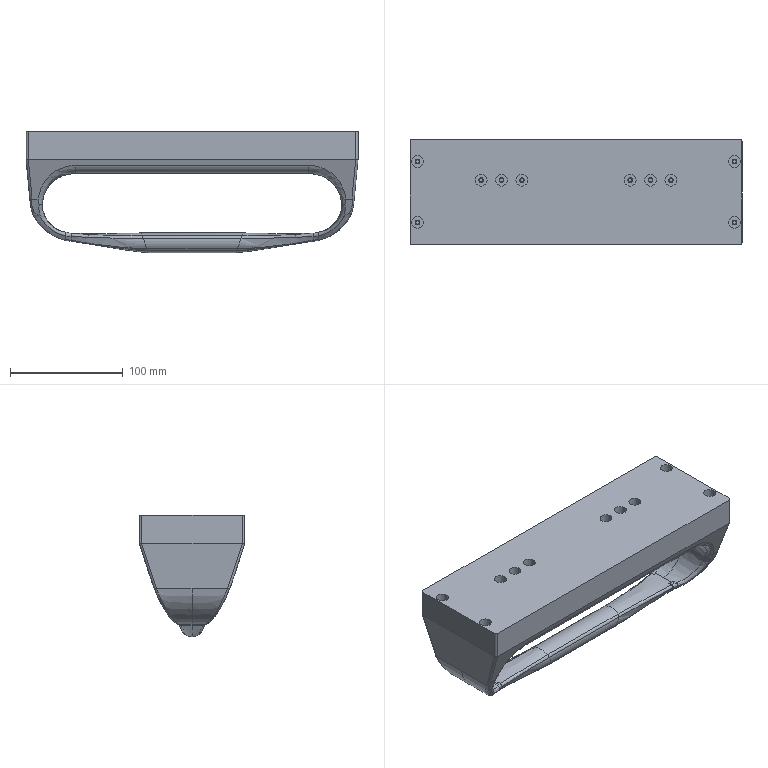NC program | NX | posted with a generic post | part box 294.078 x 93.5 x 107.5 mm
Lines 45094 to 46059 of 236164:
(FIXED_CONTOUR_COPY_1 , TOOL : D10R2)
N90174 T09 M6
N90176 G54
N90178 G17 G0 G90 X-46.64 Y88.562 B0. C0. S7500 M3
N90180 G43 Z30. H9
N90182 Z-38.
N90184 G94 G1 Z-40.127 F1000.
N90186 X-46.509 Y88.432 Z-40.777
N90188 X-46.127 Y88.156 Z-41.267
N90190 X-45.588 Y87.879 Z-41.58
N90192 X-44.971 Y87.652 Z-41.768
N90194 X-44.317 Y87.48 Z-41.871
N90196 X-43.645 Y87.358 Z-41.916
N90198 X-42.965 Y87.277 Z-41.919
N90200 X-42.283 Y87.233 Z-41.892
N90202 X-41.6 Y87.219 Z-41.84
N90204 X-40.951 Z-41.787 F2500.
N90206 X-40.435 Z-41.757
N90208 X-39.803 Z-41.736
N90210 X-39.171 Z-41.729
N90212 X-20.214 Y87.22 Z-41.732
N90214 X39.184 Y87.222 Z-41.734
N90216 X39.816 Z-41.738
N90218 X40.448 Z-41.758
N90220 X40.953 Z-41.787
N90222 X41.616 Z-41.838
N90224 X42.346 Y87.189 Z-41.847
N90226 X42.58 Y87.175 Z-41.85
N90228 X42.342 Z-41.819
N90230 X41.71 Z-41.756
N90232 X41.078 Z-41.708
N90234 X40.446 Z-41.671
N90236 X39.815 Z-41.652
N90238 X39.183 Z-41.648
N90240 X-17.802 Y87.173 Z-41.647
N90242 X-32.852
N90244 X-39.171 Z-41.645
N90246 X-39.875 Z-41.653
N90248 X-40.435 Z-41.671
N90250 X-41.067 Z-41.707
N90252 X-41.699 Z-41.758
N90254 X-42.402 Z-41.831
N90256 X-42.547 Z-41.85
N90258 X-42.965 Y87.147 Z-41.855
N90260 X-43.272 Y87.126 Z-41.858
N90262 X-42.962 Z-41.812
N90264 X-42.59 Z-41.763
N90266 X-42.33 Z-41.735
N90268 X-42.071 Z-41.711
N90270 X-41.699 Z-41.672
N90272 X-41.439 Z-41.655
N90274 X-41.067 Z-41.624
N90276 X-40.807 Z-41.612
N90278 X-40.435 Z-41.59
N90280 X-39.803 Z-41.571
N90282 X-39.171 Z-41.565
N90284 X-16.551 Y87.127 Z-41.567
N90286 X39.183 Y87.128 Z-41.569
N90288 X39.815 Z-41.572
N90290 X40.446 Z-41.59
N90292 X41.078 Z-41.625
N90294 X41.46 Z-41.655
N90296 X41.71 Z-41.67
N90298 X42.092 Z-41.709
N90300 X42.345 Z-41.732
N90302 X42.724 Z-41.78
N90304 X42.977 Z-41.808
N90306 X43.224 Z-41.839
N90308 X43.331 Z-41.857
N90310 X43.844 Y87.093 Z-41.861
N90312 X43.976 Y87.084 Z-41.862
N90314 X43.609 Z-41.808
N90316 X43.404 Z-41.774
N90318 X42.976 Z-41.719
N90320 X42.544 Z-41.672
N90322 X42.344 Z-41.647
N90324 X41.912 Z-41.608
N90326 X41.71 Z-41.587
N90328 X41.28 Z-41.561
N90330 X41.078 Z-41.546
N90332 X40.446 Z-41.511
N90334 X39.815 Z-41.495
N90336 X39.183 Z-41.492
N90338 X19.594 Y87.083
N90340 X-39.171 Y87.081 Z-41.488
N90342 X-39.803 Z-41.495
N90344 X-40.435 Z-41.513
N90346 X-40.627 Z-41.524
N90348 X-41.067 Z-41.544
N90350 X-41.259 Z-41.56
N90352 X-41.699 Z-41.589
N90354 X-41.891 Z-41.609
N90356 X-42.33 Z-41.65
N90358 X-42.77 Z-41.698
N90360 X-42.962 Z-41.723
N90362 X-43.154 Z-41.751
N90364 X-43.594 Z-41.81
N90366 X-43.943 Z-41.861
N90368 X-44.534 Y87.038 Z-41.864
N90370 X-44.208 Z-41.812
N90372 X-43.594 Z-41.722
N90374 X-42.943 Z-41.634
N90376 X-42.33 Z-41.568
N90378 X-41.699 Z-41.51
N90380 X-41.067 Z-41.468
N90382 X-40.435 Z-41.438
N90384 X-39.803 Z-41.421
N90386 X-39.171 Z-41.415
N90388 X18.969 Y87.04 Z-41.418
N90390 X33.812 Z-41.419
N90392 X39.183 Z-41.418
N90394 X39.843 Z-41.422
N90396 X40.446 Z-41.436
N90398 X41.107 Z-41.471
N90400 X41.739 Y87.041 Z-41.51
N90402 X42.37 Z-41.569
N90404 X42.974 Z-41.634
N90406 X43.606 Z-41.716
N90408 X44.239 Z-41.81
N90410 X44.585 Z-41.865
N90412 X45.158 Y86.996 Z-41.867
N90414 X45.02 Z-41.842
N90416 X44.389 Z-41.743
N90418 X44.087 Z-41.703
N90420 X43.606 Z-41.632
N90422 X43.455 Z-41.615
N90424 X42.974 Z-41.554
N90426 X42.823 Z-41.54
N90428 X42.342 Z-41.487
N90430 X41.71 Z-41.432
N90432 X41.078 Z-41.395
N90434 X40.446 Z-41.363
N90436 X39.815 Z-41.35
N90438 X39.183 Z-41.347
N90440 X21.012 Y86.995
N90442 X-39.171 Y86.994 Z-41.344
N90444 X-39.803 Z-41.349
N90446 X-40.435 Z-41.365
N90448 X-41.067 Y86.993 Z-41.393
N90450 X-41.699 Z-41.434
N90452 X-42.17 Z-41.477
N90454 X-42.33 Z-41.49
N90456 X-42.801 Z-41.541
N90458 X-42.962 Z-41.556
N90460 X-43.433 Z-41.619
N90462 X-43.755 Z-41.657
N90464 X-44.226 Z-41.726
N90466 X-44.697 Z-41.802
N90468 X-45.019 Z-41.851
N90470 X-45.107 Z-41.867
N90472 X-45.626 Y86.949 Z-41.869
N90474 X-45.196 Z-41.789
N90476 X-44.858 Z-41.736
N90478 X-44.52 Z-41.687
N90480 X-44.226 Z-41.639
N90482 X-43.932 Z-41.596
N90484 X-43.256 Z-41.516
N90486 X-42.962 Z-41.477
N90488 X-42.624 Z-41.446
N90490 X-42.33 Z-41.414
N90492 X-41.993 Z-41.387
N90494 X-41.699 Z-41.36
N90496 X-41.067 Z-41.321
N90498 X-40.729 Z-41.308
N90500 X-40.435 Y86.95 Z-41.294
N90502 X-39.803 Z-41.279
N90504 X-39.171 Z-41.274
N90506 X39.511 Y86.952 Z-41.279
N90508 X39.815 Z-41.28
N90510 X40.446 Z-41.292
N90512 X41.407 Z-41.34
N90514 X41.71 Z-41.358
N90516 X42.014 Z-41.385
N90518 X42.342 Z-41.412
N90520 X42.646 Z-41.445
N90522 X42.974 Z-41.475
N90524 X43.278 Z-41.514
N90526 X43.606 Z-41.55
N90528 X43.91 Z-41.595
N90530 X44.238 Z-41.636
N90532 X44.566 Z-41.682
N90534 X45.197 Z-41.78
N90536 X45.677 Z-41.869
N90538 X46.163 Y86.909
N90540 X45.369 Z-41.72
N90542 X44.738 Z-41.623
N90544 X44.238 Z-41.553
N90546 X43.738 Z-41.49
N90548 X43.606 Z-41.471
N90550 X43.106 Z-41.416
N90552 X42.974 Z-41.399
N90554 X42.474 Z-41.353
N90556 X42.342 Z-41.338
N90558 X41.71 Z-41.286
N90560 X41.078 Z-41.252
N90562 X40.446 Z-41.223
N90564 X39.815 Z-41.212
N90566 X39.183 Z-41.21
N90568 X-39.293 Y86.907 Z-41.208
N90570 X-39.803 Z-41.211
N90572 X-40.435 Z-41.225
N90574 X-41.067 Z-41.25
N90576 X-41.699 Z-41.289
N90578 X-42.33 Z-41.341
N90580 X-42.452 Z-41.354
N90582 X-42.962 Z-41.4
N90584 X-43.084 Z-41.417
N90586 X-44.104 Z-41.537
N90588 X-44.348 Z-41.575
N90590 X-44.858 Z-41.649
N90592 X-45.368 Z-41.729
N90594 X-46.121 Z-41.872
N90596 X-46.44 Y86.882
N90598 X-46.618 Y86.864 Z-41.869
N90600 X-46.463 Z-41.836
N90602 X-46.122 Z-41.78
N90604 X-45.541 Z-41.669
N90606 X-44.858 Z-41.564
N90608 X-44.226 Z-41.473
N90610 X-43.594 Z-41.398
N90612 X-43.013 Z-41.33
N90614 X-42.33 Z-41.268
N90616 X-41.699 Z-41.219
N90618 X-41.067 Z-41.182
N90620 X-40.384 Z-41.157
N90622 X-39.803 Z-41.145
N90624 X-39.171 Z-41.14
N90626 X39.183 Y86.866 Z-41.144
N90628 X39.815 Z-41.145
N90630 X40.446 Z-41.155
N90632 X41.119 Z-41.185
N90634 X41.751 Z-41.219
N90636 X42.383 Z-41.269
N90638 X43.015 Z-41.328
N90640 X43.647 Z-41.397
N90642 X44.278 Z-41.476
N90644 X44.91 Z-41.564
N90646 X45.542 Z-41.66
N90648 X46.133 Z-41.772
N90650 X46.47 Z-41.829
N90652 X46.656 Z-41.868
N90654 X46.77 Y86.856
N90656 X47.032 Y86.825 Z-41.846
N90658 X46.769 Z-41.799
N90660 X46.553 Z-41.754
N90662 X46.133 Z-41.683
N90664 X45.71 Z-41.603
N90666 X45.502 Z-41.573
N90668 X45.078 Z-41.509
N90670 X44.446 Z-41.421
N90672 X43.814 Z-41.342
N90674 X43.182 Z-41.274
N90676 X42.551 Z-41.216
N90678 X41.919 Z-41.167
N90680 X41.71 Z-41.153
N90682 X41.287 Z-41.13
N90684 X40.446 Y86.824 Z-41.095
N90686 X39.815 Z-41.085
N90688 X39.183 Z-41.083
N90690 X-39.171 Y86.822 Z-41.079
N90692 X-39.803 Z-41.084
N90694 X-40.435 Z-41.098
N90696 X-40.849 Z-41.114
N90698 X-41.067 Z-41.12
N90700 X-41.285 Z-41.131
N90702 X-41.917 Z-41.169
N90704 X-42.549 Z-41.219
N90706 X-43.181 Z-41.277
N90708 X-43.594 Z-41.325
N90710 X-43.813 Z-41.347
N90712 X-44.445 Z-41.424
N90714 X-45.077 Z-41.516
N90716 X-45.49 Z-41.581
N90718 X-45.709 Z-41.612
N90720 X-46.122 Z-41.691
N90722 X-46.547 Z-41.761
N90724 X-46.754 Z-41.805
N90726 X-47.021 Z-41.855
N90728 X-47.19 Y86.792 Z-41.82
N90730 X-46.754 Z-41.737
N90732 X-46.608 Z-41.707
N90734 X-46.122 Z-41.627
N90736 X-45.83 Z-41.571
N90738 X-45.49 Z-41.522
N90740 X-45.198 Z-41.476
N90742 X-44.566 Z-41.385
N90744 X-43.934 Z-41.307
N90746 X-43.594 Z-41.272
N90748 X-43.302 Z-41.238
N90750 X-42.67 Z-41.18
N90752 X-42.038 Z-41.131
N90754 X-41.406 Z-41.092
N90756 X-41.067 Z-41.075
N90758 X-40.727 Z-41.066
N90760 X-40.435 Z-41.054
N90762 X-39.803 Z-41.04
N90764 X-39.171 Z-41.035
N90766 X39.183 Y86.794 Z-41.039
N90768 X39.815 Z-41.041
N90770 X40.446 Z-41.051
N90772 X41.408 Z-41.091
N90774 X41.71 Z-41.107
N90776 X42.04 Z-41.129
N90778 X42.672 Z-41.177
N90780 X43.304 Z-41.235
N90782 X43.936 Z-41.302
N90784 X44.567 Z-41.381
N90786 X45.199 Z-41.468
N90788 X45.502 Z-41.515
N90790 X45.831 Z-41.561
N90792 X46.133 Z-41.619
N90794 X46.614 Z-41.7
N90796 X46.768 Z-41.732
N90798 X47.236 Y86.795 Z-41.816
N90800 X47.41 Y86.765 Z-41.787
N90802 X47.305 Z-41.763
N90804 X46.767 Z-41.667
N90806 X46.673 Z-41.647
N90808 X46.133 Z-41.555
N90810 X45.95 Z-41.521
N90812 X45.502 Z-41.457
N90814 X45.318 Z-41.429
N90816 X44.686 Z-41.342
N90818 X44.054 Z-41.264
N90820 X43.423 Z-41.197
N90822 X42.791 Z-41.14
N90824 X42.159 Z-41.092
N90826 X41.71 Z-41.062
N90828 X41.527 Z-41.052
N90830 X40.446 Z-41.008
N90832 X39.815 Z-40.998
N90834 X39.183 Z-40.996
N90836 X-39.171 Y86.762 Z-40.992
N90838 X-39.803 Z-40.996
N90840 X-40.435 Z-41.012
N90842 X-40.608 Z-41.019
N90844 X-41.067 Z-41.032
N90846 X-41.525 Z-41.054
N90848 X-42.157 Z-41.094
N90850 X-42.789 Z-41.142
N90852 X-43.421 Z-41.201
N90854 X-43.594 Z-41.221
N90856 X-44.053 Z-41.267
N90858 X-44.685 Z-41.346
N90860 X-45.317 Z-41.437
N90862 X-45.49 Z-41.464
N90864 X-45.949 Z-41.531
N90866 X-46.122 Z-41.564
N90868 X-46.667 Z-41.653
N90870 X-46.754 Z-41.672
N90872 X-47.299 Z-41.775
N90874 X-47.354 Z-41.787
N90876 X-47.513 Y86.735 Z-41.756
N90878 X-47.355 Z-41.724
N90880 X-46.723 Z-41.604
N90882 X-46.122 Z-41.505
N90884 X-46.06 Z-41.493
N90886 X-44.796 Z-41.31
N90888 X-44.164 Z-41.23
N90890 X-43.532 Z-41.166
N90892 X-42.9 Z-41.107
N90894 X-42.268 Z-41.059
N90896 X-41.636 Z-41.018
N90898 X-41.067 Z-40.991
N90900 X-39.803 Z-40.956
N90902 X-39.171 Z-40.952
N90904 X39.183 Y86.737 Z-40.956
N90906 X39.815 Z-40.958
N90908 X40.446 Z-40.968
N90910 X41.71 Z-41.02
N90912 X42.342 Z-41.064
N90914 X42.902 Z-41.104
N90916 X43.606 Z-41.17
N90918 X44.165 Z-41.228
N90920 X44.87 Z-41.315
N90922 X45.502 Z-41.403
N90924 X46.061 Z-41.483
N90926 X46.729 Z-41.598
N90928 X47.361 Z-41.712
N90930 X47.577 Z-41.756
N90932 X47.734 Y86.711 Z-41.726
N90934 X47.397 Z-41.66
N90936 X46.765 Z-41.548
N90938 X46.168 Z-41.446
N90940 X45.502 Z-41.353
N90942 X44.87 Z-41.267
N90944 X44.238 Z-41.19
N90946 X43.641 Z-41.128
N90948 X42.974 Z-41.068
N90950 X42.342 Z-41.022
N90952 X41.71 Z-40.981
N90954 X40.464 Z-40.931
N90956 X39.815 Z-40.92
N90958 X39.183 Y86.71 Z-40.919
N90960 X-39.171 Y86.708 Z-40.914
N90962 X-39.825 Z-40.919
N90964 X-41.089 Z-40.954
N90966 X-41.743 Z-40.985
N90968 X-42.375 Z-41.026
N90970 X-43.007 Z-41.073
N90972 X-43.639 Z-41.132
N90974 X-44.271 Z-41.196
N90976 X-44.903 Z-41.276
N90978 X-45.535 Z-41.365
N90980 X-46.167 Z-41.456
N90982 X-46.799 Z-41.56
N90984 X-47.666 Z-41.726
N90986 X-47.813 Y86.68 Z-41.695
N90988 X-47.386 Z-41.612
N90990 X-46.911 Z-41.522
N90992 X-46.279 Z-41.418
N90994 X-45.647 Z-41.328
N90996 X-45.49 Z-41.309
N90998 X-45.015 Z-41.242
N91000 X-44.226 Z-41.145
N91002 X-43.751 Z-41.097
N91004 X-43.119 Z-41.039
N91006 X-42.487 Z-40.991
N91008 X-41.855 Z-40.95
N91010 X-41.699 Z-40.945
N91012 X-41.067 Z-40.915
N91014 X-39.803 Z-40.882
N91016 X-39.171 Z-40.878
N91018 X39.183 Y86.683 Z-40.882
N91020 X39.379 Z-40.88
N91022 X39.815 Z-40.881
N91024 X40.25 Z-40.888
N91026 X40.52 Z-40.896
N91028 X41.857 Z-40.948
N91030 X42.489 Z-40.99
N91032 X43.121 Z-41.036
N91034 X43.753 Z-41.094
N91036 X44.385 Z-41.16
N91038 X44.87 Z-41.22
N91040 X45.016 Z-41.236
N91042 X45.502 Z-41.303
N91044 X45.648 Z-41.319
N91046 X46.28 Z-41.409
N91048 X46.765 Z-41.491
N91050 X46.912 Z-41.515
N91052 X47.397 Z-41.602
N91054 X47.885 Z-41.697
N91056 X48.043 Y86.654 Z-41.667
N91058 X47.397 Z-41.541
N91060 X47.027 Z-41.475
N91062 X46.765 Z-41.434
N91064 X46.395 Z-41.371
N91066 X45.763 Z-41.281
N91068 X45.502 Z-41.251
N91070 X45.131 Z-41.2
N91072 X44.87 Z-41.171
N91074 X44.499 Z-41.126
N91076 X43.868 Z-41.059
N91078 X43.236 Z-41.001
N91080 X42.604 Z-40.954
N91082 X41.972 Z-40.913
N91084 X41.209 Z-40.882
N91086 X40.446 Z-40.856
N91088 X40.097 Z-40.846
N91090 X39.815 Z-40.842
N91092 X39.532 Z-40.841
N91094 X39.183 Z-40.845
N91096 X-39.171 Y86.652 Z-40.84
N91098 X-39.803 Z-40.844
N91100 X-40.571 Z-40.863
N91102 X-41.202 Z-40.881
N91104 X-41.699 Z-40.905
N91106 X-41.97 Z-40.915
N91108 X-42.602 Z-40.955
N91110 X-43.234 Z-41.004
N91112 X-43.866 Z-41.062
N91114 X-44.226 Z-41.098
N91116 X-44.498 Z-41.129
N91118 X-44.858 Z-41.175
N91120 X-45.13 Z-41.206
N91122 X-45.49 Z-41.258
N91124 X-45.762 Z-41.29
N91126 X-46.122 Z-41.342
N91128 X-46.394 Z-41.379
N91130 X-47.026 Z-41.483
N91132 X-47.745 Z-41.621
N91134 X-47.961 Z-41.664
N91136 X-48.111 Y86.624 Z-41.631
N91138 X-48.017 Z-41.616
N91140 X-47.386 Z-41.492
N91142 X-47.136 Z-41.445
N91144 X-46.504 Z-41.341
N91146 X-46.122 Z-41.29
N91148 X-45.872 Z-41.253
N91150 X-45.49 Z-41.208
N91152 X-45.24 Z-41.173
N91154 X-44.858 Z-41.128
N91156 X-44.608 Z-41.097
N91158 X-44.226 Z-41.053
N91160 X-43.976 Z-41.027
N91162 X-43.344 Z-40.97
N91164 X-42.712 Z-40.921
N91166 X-42.08 Z-40.881
N91168 X-41.699 Z-40.867
N91170 X-41.258 Z-40.846
N91172 X-40.626 Z-40.827
N91174 X-39.803 Z-40.808
N91176 X-39.171 Z-40.804
N91178 X39.183 Y86.627 Z-40.808
N91180 X39.679 Z-40.803
N91182 X39.95 Z-40.806
N91184 X40.633 Z-40.824
N91186 X41.078 Z-40.842
N91188 X41.264 Z-40.847
N91190 X42.082 Z-40.879
N91192 X42.714 Z-40.919
N91194 X43.346 Z-40.967
N91196 X43.978 Z-41.025
N91198 X44.61 Z-41.093
N91200 X44.87 Z-41.125
N91202 X45.241 Z-41.166
N91204 X45.502 Z-41.202
N91206 X45.873 Z-41.244
N91208 X46.505 Z-41.334
N91210 X46.765 Z-41.378
N91212 X47.137 Z-41.437
N91214 X47.397 Z-41.484
N91216 X48.029 Z-41.606
N91218 X48.205 Z-41.635
N91220 X48.36 Y86.599 Z-41.605
N91222 X48.271 Z-41.586
N91224 X48.029 Z-41.546
N91226 X47.397 Z-41.424
N91228 X47.25 Z-41.398
N91230 X46.765 Z-41.321
N91232 X46.618 Z-41.296
N91234 X45.986 Z-41.207
N91236 X45.502 Z-41.152
N91238 X45.354 Z-41.131
N91240 X44.87 Z-41.077
N91242 X44.723 Z-41.059
N91244 X44.091 Z-40.991
N91246 X43.459 Z-40.932
N91248 X42.827 Z-40.884
N91250 X42.195 Z-40.844
N91252 X41.321 Z-40.811
N91254 X41.078 Z-40.804
N91256 X40.689 Z-40.789
N91258 X39.815 Z-40.765
N91260 X39.183 Z-40.771
N91262 X-39.171 Y86.596 Z-40.768
N91264 X-39.803 Z-40.771
N91266 X-40.05 Z-40.775
N91268 X-41.067 Z-40.802
N91270 X-41.314 Z-40.81
N91272 X-41.699 Z-40.829
N91274 X-42.194 Z-40.846
N91276 X-42.962 Z-40.896
N91278 X-43.457 Z-40.935
N91280 X-44.226 Z-41.006
N91282 X-45.353 Z-41.138
N91284 X-45.49 Z-41.158
N91286 X-45.985 Z-41.216
N91288 X-46.617 Z-41.303
N91290 X-47.249 Z-41.406
N91292 X-48.017 Z-41.556
N91294 X-48.27 Z-41.596
N91296 X-48.425 Y86.567 Z-41.564
N91298 X-48.324 Z-41.542
N91300 X-48.017 Z-41.495
N91302 X-47.366 Z-41.366
N91304 X-46.734 Z-41.263
N91306 X-46.102 Z-41.177
N91308 X-44.226 Z-40.958
N91310 X-43.574 Z-40.9
N91312 X-42.942 Z-40.849
N91314 X-42.31 Z-40.81
N91316 X-41.699 Z-40.789
N91318 X-41.372 Z-40.773
N91320 X-40.741 Z-40.753
N91322 X-40.109 Z-40.738
N91324 X-39.803 Z-40.733
N91326 X-39.171 Z-40.73
N91328 X39.183 Y86.57 Z-40.733
N91330 X39.815 Z-40.727
N91332 X40.747 Z-40.752
N91334 X41.078 Z-40.765
N91336 X41.379 Z-40.773
N91338 X42.342 Z-40.811
N91340 X42.974 Z-40.85
N91342 X43.576 Z-40.897
N91344 X44.238 Z-40.959
N91346 X45.502 Z-41.1
N91348 X46.103 Z-41.168
N91350 X46.765 Z-41.263
N91352 X47.397 Z-41.363
N91354 X48.029 Z-41.485
N91356 X48.33 Z-41.534
N91358 X48.519 Z-41.575
N91360 X48.684 Y86.54 Z-41.544
N91362 X48.389 Z-41.481
N91364 X48.032 Z-41.423
N91366 X47.485 Z-41.318
N91368 X47.31 Z-41.293
N91370 X46.765 Z-41.207
N91372 X46.221 Z-41.13
N91374 X44.958 Z-40.988
N91376 X44.87 Z-40.981
N91378 X44.326 Z-40.921
N91380 X44.15 Z-40.907
N91382 X43.606 Z-40.856
N91384 X42.974 Z-40.808
N91386 X42.254 Z-40.766
N91388 X41.438 Z-40.735
N91390 X41.078 Z-40.725
N91392 X40.807 Z-40.714
N91394 X39.815 Z-40.689
N91396 X39.183 Z-40.695
N91398 X-39.171 Y86.538 Z-40.691
N91400 X-39.803 Z-40.694
N91402 X-40.168 Z-40.7
N91404 X-41.067 Z-40.723
N91406 X-41.432 Z-40.735
N91408 X-41.699 Z-40.748
N91410 X-42.33 Z-40.771
N91412 X-42.962 Z-40.81
N91414 X-43.496 Z-40.852
N91416 X-43.692 Z-40.866
N91418 X-44.324 Z-40.922
N91420 X-44.858 Z-40.984
N91422 X-44.956 Z-40.992
N91424 X-46.023 Z-41.117
N91426 X-46.122 Z-41.127
N91428 X-46.655 Z-41.199
N91430 X-46.754 Z-41.211
N91432 X-47.287 Z-41.298
N91434 X-47.484 Z-41.327
N91436 X-48.017 Z-41.432
N91438 X-48.383 Z-41.489
N91440 X-48.595 Z-41.534
N91442 X-48.768 Y86.511 Z-41.509
N91444 X-48.649 Z-41.486
N91446 X-48.436 Z-41.441
N91448 X-48.017 Z-41.376
N91450 X-47.59 Z-41.291
N91452 X-47.181 Z-41.231
N91454 X-46.754 Z-41.162
N91456 X-46.549 Z-41.138
N91458 X-46.122 Z-41.08
N91460 X-45.917 Z-41.06
N91462 X-45.063 Z-40.96
N91464 X-44.858 Z-40.941
N91466 X-44.431 Z-40.892
N91468 X-43.799 Z-40.835
N91470 X-43.39 Z-40.807
N91472 X-42.962 Z-40.773
N91474 X-42.758 Z-40.763
N91476 X-42.33 Z-40.736
N91478 X-42.126 Z-40.726
N91480 X-41.699 Z-40.712
N91482 X-41.485 Z-40.701
N91484 X-40.853 Z-40.681
N91486 X-40.221 Z-40.666
N91488 X-39.803 Z-40.659
N91490 X-39.171 Z-40.656
N91492 X39.183 Y86.514 Z-40.66
N91494 X39.62 Z-40.655
N91496 X39.815
N91498 X40.097 Z-40.66
N91500 X40.86 Z-40.681
N91502 X41.078 Z-40.689
N91504 X41.492 Z-40.701
N91506 X42.148 Z-40.726
N91508 X42.342 Z-40.735
N91510 X42.78 Z-40.762
N91512 X42.974 Z-40.772
N91514 X43.412 Z-40.806
N91516 X43.606 Z-40.819
N91518 X44.044 Z-40.86
N91520 X44.432 Z-40.891
N91522 X44.87 Z-40.939
N91524 X45.064 Z-40.956
N91526 X45.939 Z-41.054
N91528 X46.133 Z-41.073
N91530 X46.327 Z-41.096
N91532 X46.765 Z-41.158
N91534 X47.203 Z-41.227
N91536 X47.591 Z-41.282
N91538 X48.031 Z-41.367
N91540 X48.442 Z-41.434
N91542 X48.661 Z-41.481
N91544 X48.859 Z-41.517
N91546 X49.029 Y86.488 Z-41.491
N91548 X48.664 Z-41.424
N91550 X48.493 Z-41.388
N91552 X48.031 Z-41.312
N91554 X47.694 Z-41.248
N91556 X47.1 Z-41.164
N91558 X46.765 Z-41.111
N91560 X46.43 Z-41.063
N91562 X46.133 Z-41.027
N91564 X45.836 Z-40.999
N91566 X45.167 Z-40.924
N91568 X44.87 Z-40.898
N91570 X44.535 Z-40.861
N91572 X44.238 Z-40.836
N91574 X43.941 Z-40.814
N91576 X43.606 Z-40.783
N91578 X43.309 Z-40.763
N91580 X42.974 Z-40.737
N91582 X42.677 Z-40.722
N91584 X42.342 Z-40.701
N91586 X42.045 Z-40.687
N91588 X41.543 Z-40.668
N91590 X41.078 Z-40.655
N91592 X40.911 Z-40.648
N91594 X40.112 Z-40.627
N91596 X39.815 Z-40.623
N91598 X39.517
N91600 X39.183 Z-40.626
N91602 X-39.334 Y86.486 Z-40.624
N91604 X-39.803 Z-40.625
N91606 X-40.435 Z-40.638
N91608 X-41.067 Z-40.652
N91610 X-41.536 Z-40.668
N91612 X-41.699 Z-40.676
N91614 X-42.023 Z-40.687
N91616 X-42.33 Z-40.702
N91618 X-42.655 Z-40.722
N91620 X-42.962 Z-40.738
N91622 X-43.287 Z-40.764
N91624 X-43.902 Z-40.806
N91626 X-44.534 Z-40.863
N91628 X-44.858 Z-40.9
N91630 X-45.166 Z-40.928
N91632 X-45.814 Z-41.004
N91634 X-46.122 Z-41.034
N91636 X-46.446 Z-41.078
N91638 X-46.754 Z-41.114
N91640 X-47.078 Z-41.167
N91642 X-47.386 Z-41.211
N91644 X-47.693 Z-41.257
N91646 X-48.017 Z-41.321
N91648 X-48.486 Z-41.394
N91650 X-48.649 Z-41.429
N91652 X-48.938 Z-41.484
N91654 X-49.106 Y86.461 Z-41.459
N91656 X-48.649 Z-41.372
N91658 X-48.537 Z-41.348
N91660 X-48.017 Z-41.268
N91662 X-47.794 Z-41.224
N91664 X-47.386 Z-41.162
N91666 X-46.977 Z-41.104
N91668 X-46.754 Z-41.067
N91670 X-46.345 Z-41.019
N91672 X-46.122 Z-40.989
N91674 X-45.713 Z-40.949
N91676 X-45.266 Z-40.897
N91678 X-44.858 Z-40.86
N91680 X-44.635 Z-40.834
N91682 X-44.003 Z-40.777
N91684 X-43.186 Z-40.721
N91686 X-42.962 Z-40.704
N91688 X-42.554 Z-40.683
N91690 X-42.33 Z-40.668
N91692 X-41.922 Z-40.649
N91694 X-41.067 Z-40.619
N91696 X-40.323 Z-40.601
N91698 X-39.803 Z-40.592
N91700 X-39.171 Z-40.59
N91702 X39.183 Y86.463 Z-40.593
N91704 X39.416 Z-40.591
N91706 X39.815
N91708 X40.26 Z-40.598
N91710 X41.594 Z-40.635
N91712 X41.944 Z-40.649
N91714 X42.342 Z-40.668
N91716 X42.576 Z-40.682
N91718 X42.974 Z-40.703
N91720 X43.208 Z-40.721
N91722 X43.606 Z-40.747
N91724 X43.84 Z-40.769
N91726 X44.238 Z-40.798
N91728 X44.636 Z-40.832
N91730 X44.87 Z-40.858
N91732 X45.268 Z-40.893
N91734 X45.735 Z-40.945
N91736 X46.133 Z-40.983
N91738 X46.531 Z-41.031
N91740 X46.765 Z-41.064
N91742 X46.999 Z-41.101
N91744 X47.795 Z-41.214
N91746 X48.03 Z-41.259
N91748 X48.544 Z-41.343
N91750 X48.663 Z-41.368
N91752 X49.193 Z-41.466
N91754 X49.354 Y86.438 Z-41.442
N91756 X49.228 Z-41.414
N91758 X48.662 Y86.437 Z-41.31
N91760 X48.596 Z-41.296
N91762 X48.03 Z-41.204
N91764 X47.899 Z-41.179
N91766 X47.397 Z-41.106
N91768 X46.895 Z-41.037
N91770 X46.635 Z-40.998
N91772 X46.133 Z-40.937
N91774 X45.632 Z-40.89
N91776 X45.372 Z-40.861
N91778 X44.87 Z-40.817
N91780 X44.74 Z-40.803
N91782 X44.238 Z-40.76
N91784 X43.736 Z-40.723
N91786 X43.606 Z-40.711
N91788 X43.104 Z-40.678
N91790 X42.974 Z-40.668
N91792 X42.342 Z-40.634
N91794 X41.71 Z-40.605
N91796 X41.014 Z-40.584
N91798 X40.317 Z-40.565
N91800 X39.815 Z-40.558
N91802 X-39.231 Y86.435 Z-40.557
N91804 X-39.803 Z-40.558
N91806 X-41.007 Z-40.582
N91808 X-41.818 Z-40.61
N91810 X-42.33 Z-40.634
N91812 X-42.962 Z-40.668
N91814 X-44.106 Z-40.748
N91816 X-44.738 Z-40.805
N91818 X-44.858 Z-40.818
N91820 X-45.37 Z-40.865
N91822 X-45.609 Z-40.893
N91824 X-46.122 Z-40.943
N91826 X-46.241 Z-40.959
N91828 X-46.754 Z-41.019
N91830 X-46.873 Z-41.039
N91832 X-47.386 Z-41.112
N91834 X-47.898 Z-41.189
N91836 X-48.017 Z-41.213
N91838 X-48.589 Z-41.301
N91840 X-48.649 Z-41.314
N91842 X-49.222 Z-41.423
N91844 X-49.273 Z-41.434
N91846 X-49.439 Y86.409 Z-41.411
N91848 X-49.274 Z-41.374
N91850 X-48.642 Z-41.255
N91852 X-48.002 Z-41.155
N91854 X-47.386 Z-41.061
N91856 X-46.754 Z-40.971
N91858 X-46.122 Z-40.896
N91860 X-45.474 Z-40.833
N91862 X-44.211 Z-40.718
N91864 X-42.962 Z-40.633
N91866 X-42.33 Z-40.6
N91868 X-41.691 Z-40.57
N91870 X-41.059 Z-40.548
N91872 X-39.803 Z-40.524
N91874 X-39.171 Z-40.522
N91876 X39.815 Y86.411 Z-40.525
N91878 X40.426 Z-40.534
N91880 X41.736 Z-40.57
N91882 X42.974 Z-40.632
N91884 X43.632 Z-40.676
N91886 X44.238 Z-40.721
N91888 X45.476 Y86.412 Z-40.828
N91890 X46.133 Z-40.892
N91892 X46.765 Z-40.969
N91894 X47.397 Z-41.056
N91896 X48.029 Z-41.149
N91898 X48.661 Z-41.253
N91900 X49.294 Z-41.369
N91902 X49.52 Z-41.418
N91904 X49.686 Y86.385 Z-41.393
N91906 X49.373 Z-41.326
N91908 X48.741 Z-41.21
N91910 X48.109 Z-41.108
N91912 X47.477 Z-41.018
N91914 X47.397 Z-41.01
N91916 X46.805 Z-40.928
N91918 X46.133 Z-40.849
N91920 X45.502 Z-40.79
N91922 X44.238 Z-40.683
N91924 X43.606 Z-40.637
N91926 X42.974 Z-40.597
N91928 X41.791 Z-40.538
N91930 X40.446 Z-40.503
N91932 X39.815 Z-40.494
N91934 X-39.803 Y86.383 Z-40.491
N91936 X-40.435 Z-40.504
N91938 X-41.112 Z-40.518
N91940 X-41.699 Z-40.538
N91942 X-42.33 Z-40.567
N91944 X-42.421 Z-40.569
N91946 X-42.962 Z-40.597
N91948 X-43.594 Z-40.639
N91950 X-44.317 Z-40.689
N91952 X-45.581 Z-40.802
N91954 X-46.213 Z-40.864
N91956 X-46.844 Y86.382 Z-40.938
N91958 X-47.386 Z-41.015
N91960 X-47.476 Z-41.025
N91962 X-48.558 Z-41.191
N91964 X-48.649 Z-41.202
N91966 X-48.74 Z-41.217
N91968 X-49.372 Z-41.336
N91970 X-49.606 Z-41.388
N91972 X-49.777 Y86.355 Z-41.364
N91974 X-49.481 Z-41.298
N91976 X-48.849 Z-41.179
N91978 X-48.649 Z-41.148
N91980 X-48.45 Z-41.123
N91982 X-47.585 Z-40.99
N91984 X-47.386 Z-40.967
N91986 X-46.953 Z-40.906
N91988 X-46.321 Z-40.832
N91990 X-45.689 Y86.356 Z-40.77
N91992 X-44.425 Z-40.658
N91994 X-43.793 Z-40.614
N91996 X-43.395 Z-40.591
N91998 X-42.962 Z-40.561
N92000 X-42.529 Z-40.539
N92002 X-42.231 Z-40.531
N92004 X-41.699 Z-40.506
N92006 X-41.067 Z-40.485
N92008 X-40.435 Z-40.473
N92010 X-40.037 Z-40.463
N92012 X-39.803 Z-40.458
N92014 X-39.171 Z-40.46
N92016 X39.909 Y86.358 Z-40.464
N92018 X40.446 Z-40.472
N92020 X41.899 Z-40.509
N92022 X42.785 Z-40.553
N92024 X42.974 Z-40.561
N92026 X43.417 Z-40.59
N92028 X43.606 Z-40.6
N92030 X44.049 Z-40.633
N92032 X44.427 Z-40.658
N92034 X45.502 Z-40.749
N92036 X45.945 Z-40.791
N92038 X46.133 Z-40.807
N92040 X46.322 Z-40.828
N92042 X46.765 Z-40.881
N92044 X46.954 Z-40.902
N92046 X47.397 Z-40.963
N92048 X47.586 Z-40.984
N92050 X48.029 Z-41.048
N92052 X48.218 Z-41.072
N92054 X48.849 Z-41.173
N92056 X49.481 Z-41.288
N92058 X49.855 Z-41.368
N92060 X50.029 Y86.332 Z-41.343
N92062 X49.925 Z-41.323
N92064 X49.588 Z-41.251
N92066 X48.956 Z-41.136
N92068 X48.661 Z-41.091
N92070 X48.324 Z-41.036
N92072 X48.029 Z-40.998
N92074 X47.692 Z-40.95
N92076 X47.397 Z-40.917
N92078 X47.061 Z-40.871
N92080 X46.913 Z-40.853
N92082 X46.765 Z-40.838
N92084 X46.429 Z-40.798
N92086 X46.133 Z-40.766
N92088 X45.838 Z-40.741
N92090 X45.502 Z-40.709
N92092 X44.533 Z-40.628
N92094 X44.238 Z-40.606
N92096 X43.942 Z-40.588
N92098 X43.606 Z-40.563